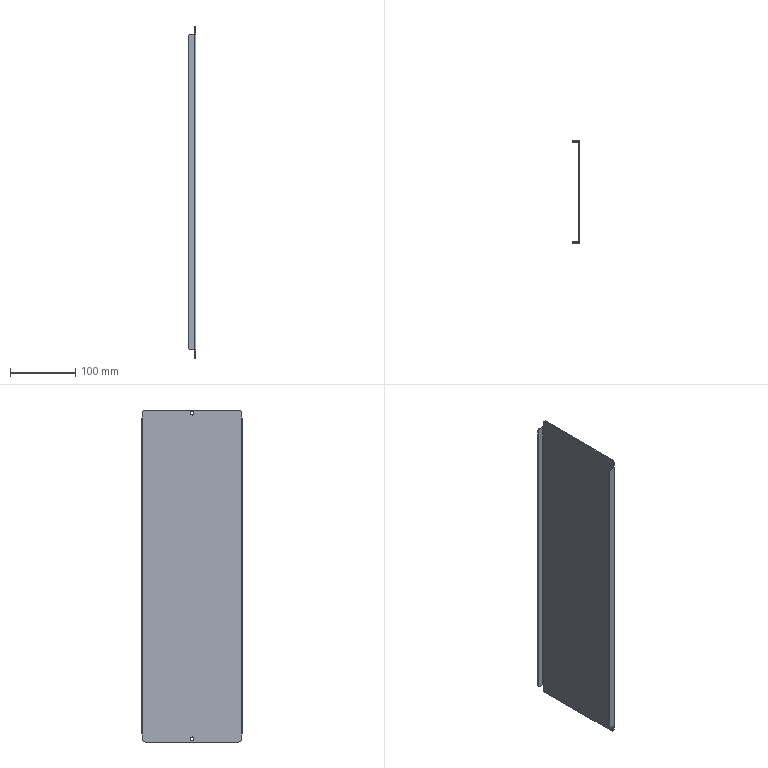Part | SolidWorks | 1 solid | 38 faces | box 12 x 156.2 x 510 mm | volume 133984 mm3 | plane 22 | cylinder 16 | commonest cylinder face diameters 10 x8 5.5 x4 0.2 x2 3.2 x2
STEP:
#1=CARTESIAN_POINT('',(-1.5,0.,247.25));
#2=VERTEX_POINT('',#1);
#3=CARTESIAN_POINT('',(-1.5,0.,252.75));
#4=VERTEX_POINT('',#3);
#5=CARTESIAN_POINT('',(-1.5,0.,250.));
#6=DIRECTION('',(-1.,0.,0.));
#7=DIRECTION('',(0.,0.,-1.));
#8=AXIS2_PLACEMENT_3D('',#5,#6,#7);
#9=CIRCLE('',#8,2.75);
#10=EDGE_CURVE('',#2,#4,#9,.T.);
#11=ORIENTED_EDGE('',*,*,#10,.T.);
#12=CARTESIAN_POINT('',(0.,0.,252.75));
#13=VERTEX_POINT('',#12);
#14=CARTESIAN_POINT('',(-12.001,0.,252.75));
#15=DIRECTION('',(1.,0.,0.));
#16=VECTOR('',#15,1000.);
#17=LINE('',#14,#16);
#18=EDGE_CURVE('',#4,#13,#17,.T.);
#19=ORIENTED_EDGE('',*,*,#18,.T.);
#20=CARTESIAN_POINT('',(0.,0.,247.25));
#21=VERTEX_POINT('',#20);
#22=CARTESIAN_POINT('',(0.,0.,250.));
#23=DIRECTION('',(1.,0.,0.));
#24=DIRECTION('',(0.,0.,-1.));
#25=AXIS2_PLACEMENT_3D('',#22,#23,#24);
#26=CIRCLE('',#25,2.75);
#27=EDGE_CURVE('',#13,#21,#26,.T.);
#28=ORIENTED_EDGE('',*,*,#27,.T.);
#29=CARTESIAN_POINT('',(-12.001,0.,247.25));
#30=DIRECTION('',(1.,0.,0.));
#31=VECTOR('',#30,1000.);
#32=LINE('',#29,#31);
#33=EDGE_CURVE('',#2,#21,#32,.T.);
#34=ORIENTED_EDGE('',*,*,#33,.F.);
#35=EDGE_LOOP('',(#11,#19,#28,#34));
#36=FACE_OUTER_BOUND('',#35,.T.);
#37=CARTESIAN_POINT('',(-12.001,0.,250.));
#38=DIRECTION('',(1.,0.,0.));
#39=DIRECTION('',(0.,0.,-1.));
#40=AXIS2_PLACEMENT_3D('',#37,#38,#39);
#41=CYLINDRICAL_SURFACE('',#40,2.75);
#42=ADVANCED_FACE('',(#36),#41,.F.);
#43=CARTESIAN_POINT('',(-1.5,0.,-252.75));
#44=VERTEX_POINT('',#43);
#45=CARTESIAN_POINT('',(-1.5,0.,-247.25));
#46=VERTEX_POINT('',#45);
#47=CARTESIAN_POINT('',(-1.5,0.,-250.));
#48=DIRECTION('',(-1.,0.,0.));
#49=DIRECTION('',(0.,0.,-1.));
#50=AXIS2_PLACEMENT_3D('',#47,#48,#49);
#51=CIRCLE('',#50,2.75);
#52=EDGE_CURVE('',#44,#46,#51,.T.);
#53=ORIENTED_EDGE('',*,*,#52,.T.);
#54=CARTESIAN_POINT('',(0.,0.,-247.25));
#55=VERTEX_POINT('',#54);
#56=CARTESIAN_POINT('',(-12.001,0.,-247.25));
#57=DIRECTION('',(1.,0.,0.));
#58=VECTOR('',#57,1000.);
#59=LINE('',#56,#58);
#60=EDGE_CURVE('',#46,#55,#59,.T.);
#61=ORIENTED_EDGE('',*,*,#60,.T.);
#62=CARTESIAN_POINT('',(0.,0.,-252.75));
#63=VERTEX_POINT('',#62);
#64=CARTESIAN_POINT('',(0.,0.,-250.));
#65=DIRECTION('',(1.,0.,0.));
#66=DIRECTION('',(0.,0.,1.));
#67=AXIS2_PLACEMENT_3D('',#64,#65,#66);
#68=CIRCLE('',#67,2.75);
#69=EDGE_CURVE('',#55,#63,#68,.T.);
#70=ORIENTED_EDGE('',*,*,#69,.T.);
#71=CARTESIAN_POINT('',(-12.001,0.,-252.75));
#72=DIRECTION('',(1.,0.,0.));
#73=VECTOR('',#72,1000.);
#74=LINE('',#71,#73);
#75=EDGE_CURVE('',#44,#63,#74,.T.);
#76=ORIENTED_EDGE('',*,*,#75,.F.);
#77=EDGE_LOOP('',(#53,#61,#70,#76));
#78=FACE_OUTER_BOUND('',#77,.T.);
#79=CARTESIAN_POINT('',(-12.001,0.,-250.));
#80=DIRECTION('',(1.,0.,0.));
#81=DIRECTION('',(0.,0.,-1.));
#82=AXIS2_PLACEMENT_3D('',#79,#80,#81);
#83=CYLINDRICAL_SURFACE('',#82,2.75);
#84=ADVANCED_FACE('',(#78),#83,.F.);
#85=CARTESIAN_POINT('',(0.,-76.5,250.));
#86=VERTEX_POINT('',#85);
#87=CARTESIAN_POINT('',(0.,-76.5,242.5));
#88=VERTEX_POINT('',#87);
#89=CARTESIAN_POINT('',(0.,-76.5,-255.));
#90=DIRECTION('',(0.,0.,-1.));
#91=VECTOR('',#90,1000.);
#92=LINE('',#89,#91);
#93=EDGE_CURVE('',#86,#88,#92,.T.);
#94=ORIENTED_EDGE('',*,*,#93,.F.);
#95=CARTESIAN_POINT('',(-1.5,-76.5,250.));
#96=VERTEX_POINT('',#95);
#97=CARTESIAN_POINT('',(-1.5,-76.5,250.));
#98=DIRECTION('',(-1.,0.,0.));
#99=VECTOR('',#98,1000.);
#100=LINE('',#97,#99);
#101=EDGE_CURVE('',#86,#96,#100,.T.);
#102=ORIENTED_EDGE('',*,*,#101,.T.);
#103=CARTESIAN_POINT('',(-1.5,-76.5,242.5));
#104=VERTEX_POINT('',#103);
#105=CARTESIAN_POINT('',(-1.5,-76.5,-255.));
#106=DIRECTION('',(0.,0.,-1.));
#107=VECTOR('',#106,1000.);
#108=LINE('',#105,#107);
#109=EDGE_CURVE('',#96,#104,#108,.T.);
#110=ORIENTED_EDGE('',*,*,#109,.T.);
#111=CARTESIAN_POINT('',(-1.5,-76.5,242.5));
#112=DIRECTION('',(1.,0.,0.));
#113=VECTOR('',#112,1000.);
#114=LINE('',#111,#113);
#115=EDGE_CURVE('',#104,#88,#114,.T.);
#116=ORIENTED_EDGE('',*,*,#115,.T.);
#117=EDGE_LOOP('',(#94,#102,#110,#116));
#118=FACE_OUTER_BOUND('',#117,.T.);
#119=CARTESIAN_POINT('',(-1.5,-76.5,-255.));
#120=DIRECTION('',(0.,-1.,0.));
#121=DIRECTION('',(0.,0.,-1.));
#122=AXIS2_PLACEMENT_3D('',#119,#120,#121);
#123=PLANE('',#122);
#124=ADVANCED_FACE('',(#118),#123,.T.);
#125=CARTESIAN_POINT('',(0.,76.5,-250.));
#126=VERTEX_POINT('',#125);
#127=CARTESIAN_POINT('',(0.,76.5,-242.5));
#128=VERTEX_POINT('',#127);
#129=CARTESIAN_POINT('',(0.,76.5,-255.));
#130=DIRECTION('',(0.,0.,1.));
#131=VECTOR('',#130,1000.);
#132=LINE('',#129,#131);
#133=EDGE_CURVE('',#126,#128,#132,.T.);
#134=ORIENTED_EDGE('',*,*,#133,.F.);
#135=CARTESIAN_POINT('',(-1.5,76.5,-250.));
#136=VERTEX_POINT('',#135);
#137=CARTESIAN_POINT('',(-1.5,76.5,-250.));
#138=DIRECTION('',(-1.,0.,0.));
#139=VECTOR('',#138,1000.);
#140=LINE('',#137,#139);
#141=EDGE_CURVE('',#126,#136,#140,.T.);
#142=ORIENTED_EDGE('',*,*,#141,.T.);
#143=CARTESIAN_POINT('',(-1.5,76.5,-242.5));
#144=VERTEX_POINT('',#143);
#145=CARTESIAN_POINT('',(-1.5,76.5,-255.));
#146=DIRECTION('',(0.,0.,1.));
#147=VECTOR('',#146,1000.);
#148=LINE('',#145,#147);
#149=EDGE_CURVE('',#136,#144,#148,.T.);
#150=ORIENTED_EDGE('',*,*,#149,.T.);
#151=CARTESIAN_POINT('',(-1.5,76.5,-242.5));
#152=DIRECTION('',(1.,0.,0.));
#153=VECTOR('',#152,1000.);
#154=LINE('',#151,#153);
#155=EDGE_CURVE('',#144,#128,#154,.T.);
#156=ORIENTED_EDGE('',*,*,#155,.T.);
#157=EDGE_LOOP('',(#134,#142,#150,#156));
#158=FACE_OUTER_BOUND('',#157,.T.);
#159=CARTESIAN_POINT('',(-1.5,76.5,-255.));
#160=DIRECTION('',(0.,1.,0.));
#161=DIRECTION('',(0.,0.,1.));
#162=AXIS2_PLACEMENT_3D('',#159,#160,#161);
#163=PLANE('',#162);
#164=ADVANCED_FACE('',(#158),#163,.T.);
#165=CARTESIAN_POINT('',(0.,71.5,255.));
#166=VERTEX_POINT('',#165);
#167=CARTESIAN_POINT('',(0.,-71.5,255.));
#168=VERTEX_POINT('',#167);
#169=CARTESIAN_POINT('',(0.,-76.5,255.));
#170=DIRECTION('',(0.,-1.,0.));
#171=VECTOR('',#170,1000.);
#172=LINE('',#169,#171);
#173=EDGE_CURVE('',#166,#168,#172,.T.);
#174=ORIENTED_EDGE('',*,*,#173,.F.);
#175=CARTESIAN_POINT('',(-1.5,71.5,255.));
#176=VERTEX_POINT('',#175);
#177=CARTESIAN_POINT('',(-1.5,71.5,255.));
#178=DIRECTION('',(-1.,0.,0.));
#179=VECTOR('',#178,1000.);
#180=LINE('',#177,#179);
#181=EDGE_CURVE('',#166,#176,#180,.T.);
#182=ORIENTED_EDGE('',*,*,#181,.T.);
#183=CARTESIAN_POINT('',(-1.5,-71.5,255.));
#184=VERTEX_POINT('',#183);
#185=CARTESIAN_POINT('',(-1.5,-76.5,255.));
#186=DIRECTION('',(0.,-1.,0.));
#187=VECTOR('',#186,1000.);
#188=LINE('',#185,#187);
#189=EDGE_CURVE('',#176,#184,#188,.T.);
#190=ORIENTED_EDGE('',*,*,#189,.T.);
#191=CARTESIAN_POINT('',(-1.5,-71.5,255.));
#192=DIRECTION('',(1.,0.,0.));
#193=VECTOR('',#192,1000.);
#194=LINE('',#191,#193);
#195=EDGE_CURVE('',#184,#168,#194,.T.);
#196=ORIENTED_EDGE('',*,*,#195,.T.);
#197=EDGE_LOOP('',(#174,#182,#190,#196));
#198=FACE_OUTER_BOUND('',#197,.T.);
#199=CARTESIAN_POINT('',(-1.5,-76.5,255.));
#200=DIRECTION('',(0.,0.,1.));
#201=DIRECTION('',(1.,0.,0.));
#202=AXIS2_PLACEMENT_3D('',#199,#200,#201);
#203=PLANE('',#202);
#204=ADVANCED_FACE('',(#198),#203,.T.);
#205=CARTESIAN_POINT('',(-1.5,76.5,242.5));
#206=VERTEX_POINT('',#205);
#207=CARTESIAN_POINT('',(-1.5,76.5,250.));
#208=VERTEX_POINT('',#207);
#209=CARTESIAN_POINT('',(-1.5,76.5,-255.));
#210=DIRECTION('',(0.,0.,1.));
#211=VECTOR('',#210,1000.);
#212=LINE('',#209,#211);
#213=EDGE_CURVE('',#206,#208,#212,.T.);
#214=ORIENTED_EDGE('',*,*,#213,.T.);
#215=CARTESIAN_POINT('',(0.,76.5,250.));
#216=VERTEX_POINT('',#215);
#217=CARTESIAN_POINT('',(-1.5,76.5,250.));
#218=DIRECTION('',(1.,0.,0.));
#219=VECTOR('',#218,1000.);
#220=LINE('',#217,#219);
#221=EDGE_CURVE('',#208,#216,#220,.T.);
#222=ORIENTED_EDGE('',*,*,#221,.T.);
#223=CARTESIAN_POINT('',(0.,76.5,242.5));
#224=VERTEX_POINT('',#223);
#225=CARTESIAN_POINT('',(0.,76.5,-255.));
#226=DIRECTION('',(0.,0.,1.));
#227=VECTOR('',#226,1000.);
#228=LINE('',#225,#227);
#229=EDGE_CURVE('',#224,#216,#228,.T.);
#230=ORIENTED_EDGE('',*,*,#229,.F.);
#231=CARTESIAN_POINT('',(-1.5,76.5,242.5));
#232=DIRECTION('',(1.,0.,0.));
#233=VECTOR('',#232,1000.);
#234=LINE('',#231,#233);
#235=EDGE_CURVE('',#206,#224,#234,.T.);
#236=ORIENTED_EDGE('',*,*,#235,.F.);
#237=EDGE_LOOP('',(#214,#222,#230,#236));
#238=FACE_OUTER_BOUND('',#237,.T.);
#239=CARTESIAN_POINT('',(-1.5,76.5,-255.));
#240=DIRECTION('',(0.,1.,0.));
#241=DIRECTION('',(0.,0.,1.));
#242=AXIS2_PLACEMENT_3D('',#239,#240,#241);
#243=PLANE('',#242);
#244=ADVANCED_FACE('',(#238),#243,.T.);
#245=CARTESIAN_POINT('',(0.,-71.5,-255.));
#246=VERTEX_POINT('',#245);
#247=CARTESIAN_POINT('',(0.,71.5,-255.));
#248=VERTEX_POINT('',#247);
#249=CARTESIAN_POINT('',(0.,-76.5,-255.));
#250=DIRECTION('',(0.,1.,0.));
#251=VECTOR('',#250,1000.);
#252=LINE('',#249,#251);
#253=EDGE_CURVE('',#246,#248,#252,.T.);
#254=ORIENTED_EDGE('',*,*,#253,.F.);
#255=CARTESIAN_POINT('',(-1.5,-71.5,-255.));
#256=VERTEX_POINT('',#255);
#257=CARTESIAN_POINT('',(-1.5,-71.5,-255.));
#258=DIRECTION('',(-1.,0.,0.));
#259=VECTOR('',#258,1000.);
#260=LINE('',#257,#259);
#261=EDGE_CURVE('',#246,#256,#260,.T.);
#262=ORIENTED_EDGE('',*,*,#261,.T.);
#263=CARTESIAN_POINT('',(-1.5,71.5,-255.));
#264=VERTEX_POINT('',#263);
#265=CARTESIAN_POINT('',(-1.5,-76.5,-255.));
#266=DIRECTION('',(0.,1.,0.));
#267=VECTOR('',#266,1000.);
#268=LINE('',#265,#267);
#269=EDGE_CURVE('',#256,#264,#268,.T.);
#270=ORIENTED_EDGE('',*,*,#269,.T.);
#271=CARTESIAN_POINT('',(-1.5,71.5,-255.));
#272=DIRECTION('',(1.,0.,0.));
#273=VECTOR('',#272,1000.);
#274=LINE('',#271,#273);
#275=EDGE_CURVE('',#264,#248,#274,.T.);
#276=ORIENTED_EDGE('',*,*,#275,.T.);
#277=EDGE_LOOP('',(#254,#262,#270,#276));
#278=FACE_OUTER_BOUND('',#277,.T.);
#279=CARTESIAN_POINT('',(-1.5,-76.5,-255.));
#280=DIRECTION('',(0.,0.,-1.));
#281=DIRECTION('',(-1.,0.,0.));
#282=AXIS2_PLACEMENT_3D('',#279,#280,#281);
#283=PLANE('',#282);
#284=ADVANCED_FACE('',(#278),#283,.T.);
#285=CARTESIAN_POINT('',(-1.5,-76.5,-242.5));
#286=VERTEX_POINT('',#285);
#287=CARTESIAN_POINT('',(-1.5,-76.5,-250.));
#288=VERTEX_POINT('',#287);
#289=CARTESIAN_POINT('',(-1.5,-76.5,-255.));
#290=DIRECTION('',(0.,0.,-1.));
#291=VECTOR('',#290,1000.);
#292=LINE('',#289,#291);
#293=EDGE_CURVE('',#286,#288,#292,.T.);
#294=ORIENTED_EDGE('',*,*,#293,.T.);
#295=CARTESIAN_POINT('',(0.,-76.5,-250.));
#296=VERTEX_POINT('',#295);
#297=CARTESIAN_POINT('',(-1.5,-76.5,-250.));
#298=DIRECTION('',(1.,0.,0.));
#299=VECTOR('',#298,1000.);
#300=LINE('',#297,#299);
#301=EDGE_CURVE('',#288,#296,#300,.T.);
#302=ORIENTED_EDGE('',*,*,#301,.T.);
#303=CARTESIAN_POINT('',(0.,-76.5,-242.5));
#304=VERTEX_POINT('',#303);
#305=CARTESIAN_POINT('',(0.,-76.5,-255.));
#306=DIRECTION('',(0.,0.,-1.));
#307=VECTOR('',#306,1000.);
#308=LINE('',#305,#307);
#309=EDGE_CURVE('',#304,#296,#308,.T.);
#310=ORIENTED_EDGE('',*,*,#309,.F.);
#311=CARTESIAN_POINT('',(-1.5,-76.5,-242.5));
#312=DIRECTION('',(1.,0.,0.));
#313=VECTOR('',#312,1000.);
#314=LINE('',#311,#313);
#315=EDGE_CURVE('',#286,#304,#314,.T.);
#316=ORIENTED_EDGE('',*,*,#315,.F.);
#317=EDGE_LOOP('',(#294,#302,#310,#316));
#318=FACE_OUTER_BOUND('',#317,.T.);
#319=CARTESIAN_POINT('',(-1.5,-76.5,-255.));
#320=DIRECTION('',(0.,-1.,0.));
#321=DIRECTION('',(0.,0.,-1.));
#322=AXIS2_PLACEMENT_3D('',#319,#320,#321);
#323=PLANE('',#322);
#324=ADVANCED_FACE('',(#318),#323,.T.);
#325=ORIENTED_EDGE('',*,*,#10,.F.);
#326=CARTESIAN_POINT('',(-1.5,0.,250.));
#327=DIRECTION('',(-1.,0.,0.));
#328=DIRECTION('',(0.,0.,-1.));
#329=AXIS2_PLACEMENT_3D('',#326,#327,#328);
#330=CIRCLE('',#329,2.75);
#331=EDGE_CURVE('',#4,#2,#330,.T.);
#332=ORIENTED_EDGE('',*,*,#331,.F.);
#333=EDGE_LOOP('',(#325,#332));
#334=FACE_BOUND('',#333,.T.);
#335=ORIENTED_EDGE('',*,*,#52,.F.);
#336=CARTESIAN_POINT('',(-1.5,0.,-250.));
#337=DIRECTION('',(-1.,0.,0.));
#338=DIRECTION('',(0.,0.,-1.));
#339=AXIS2_PLACEMENT_3D('',#336,#337,#338);
#340=CIRCLE('',#339,2.75);
#341=EDGE_CURVE('',#46,#44,#340,.T.);
#342=ORIENTED_EDGE('',*,*,#341,.F.);
#343=EDGE_LOOP('',(#335,#342));
#344=FACE_BOUND('',#343,.T.);
#345=ORIENTED_EDGE('',*,*,#189,.F.);
#346=CARTESIAN_POINT('',(-1.5,71.5,250.));
#347=DIRECTION('',(-1.,0.,0.));
#348=DIRECTION('',(0.,0.,-1.));
#349=AXIS2_PLACEMENT_3D('',#346,#347,#348);
#350=CIRCLE('',#349,5.);
#351=EDGE_CURVE('',#176,#208,#350,.T.);
#352=ORIENTED_EDGE('',*,*,#351,.T.);
#353=ORIENTED_EDGE('',*,*,#213,.F.);
#354=CARTESIAN_POINT('',(-1.5,76.5,-242.5));
#355=DIRECTION('',(0.,0.,1.));
#356=VECTOR('',#355,1000.);
#357=LINE('',#354,#356);
#358=EDGE_CURVE('',#144,#206,#357,.T.);
#359=ORIENTED_EDGE('',*,*,#358,.F.);
#360=ORIENTED_EDGE('',*,*,#149,.F.);
#361=CARTESIAN_POINT('',(-1.5,71.5,-250.));
#362=DIRECTION('',(-1.,0.,0.));
#363=DIRECTION('',(0.,0.,-1.));
#364=AXIS2_PLACEMENT_3D('',#361,#362,#363);
#365=CIRCLE('',#364,5.);
#366=EDGE_CURVE('',#136,#264,#365,.T.);
#367=ORIENTED_EDGE('',*,*,#366,.T.);
#368=ORIENTED_EDGE('',*,*,#269,.F.);
#369=CARTESIAN_POINT('',(-1.5,-71.5,-250.));
#370=DIRECTION('',(-1.,0.,0.));
#371=DIRECTION('',(0.,0.,-1.));
#372=AXIS2_PLACEMENT_3D('',#369,#370,#371);
#373=CIRCLE('',#372,5.);
#374=EDGE_CURVE('',#256,#288,#373,.T.);
#375=ORIENTED_EDGE('',*,*,#374,.T.);
#376=ORIENTED_EDGE('',*,*,#293,.F.);
#377=CARTESIAN_POINT('',(-1.5,-76.5,242.5));
#378=DIRECTION('',(0.,0.,-1.));
#379=VECTOR('',#378,1000.);
#380=LINE('',#377,#379);
#381=EDGE_CURVE('',#104,#286,#380,.T.);
#382=ORIENTED_EDGE('',*,*,#381,.F.);
#383=ORIENTED_EDGE('',*,*,#109,.F.);
#384=CARTESIAN_POINT('',(-1.5,-71.5,250.));
#385=DIRECTION('',(-1.,0.,0.));
#386=DIRECTION('',(0.,0.,-1.));
#387=AXIS2_PLACEMENT_3D('',#384,#385,#386);
#388=CIRCLE('',#387,5.);
#389=EDGE_CURVE('',#96,#184,#388,.T.);
#390=ORIENTED_EDGE('',*,*,#389,.T.);
#391=EDGE_LOOP('',(#345,#352,#353,#359,#360,#367,#368,#375,#376,#382,#383,#390));
#392=FACE_OUTER_BOUND('',#391,.T.);
#393=CARTESIAN_POINT('',(-1.5,0.,0.));
#394=DIRECTION('',(1.,0.,0.));
#395=DIRECTION('',(0.,0.,-1.));
#396=AXIS2_PLACEMENT_3D('',#393,#394,#395);
#397=PLANE('',#396);
#398=ADVANCED_FACE('',(#334,#344,#392),#397,.F.);
#399=CARTESIAN_POINT('',(0.,0.,250.));
#400=DIRECTION('',(1.,0.,0.));
#401=DIRECTION('',(0.,0.,-1.));
#402=AXIS2_PLACEMENT_3D('',#399,#400,#401);
#403=CIRCLE('',#402,2.75);
#404=EDGE_CURVE('',#21,#13,#403,.T.);
#405=ORIENTED_EDGE('',*,*,#404,.F.);
#406=ORIENTED_EDGE('',*,*,#27,.F.);
#407=EDGE_LOOP('',(#405,#406));
#408=FACE_BOUND('',#407,.T.);
#409=CARTESIAN_POINT('',(0.,0.,-250.));
#410=DIRECTION('',(1.,0.,0.));
#411=DIRECTION('',(0.,0.,1.));
#412=AXIS2_PLACEMENT_3D('',#409,#410,#411);
#413=CIRCLE('',#412,2.75);
#414=EDGE_CURVE('',#63,#55,#413,.T.);
#415=ORIENTED_EDGE('',*,*,#414,.F.);
#416=ORIENTED_EDGE('',*,*,#69,.F.);
#417=EDGE_LOOP('',(#415,#416));
#418=FACE_BOUND('',#417,.T.);
#419=ORIENTED_EDGE('',*,*,#229,.T.);
#420=CARTESIAN_POINT('',(0.,71.5,250.));
#421=DIRECTION('',(1.,0.,0.));
#422=DIRECTION('',(0.,0.,-1.));
#423=AXIS2_PLACEMENT_3D('',#420,#421,#422);
#424=CIRCLE('',#423,5.);
#425=EDGE_CURVE('',#216,#166,#424,.T.);
#426=ORIENTED_EDGE('',*,*,#425,.T.);
#427=ORIENTED_EDGE('',*,*,#173,.T.);
#428=CARTESIAN_POINT('',(0.,-71.5,250.));
#429=DIRECTION('',(1.,0.,0.));
#430=DIRECTION('',(0.,0.,-1.));
#431=AXIS2_PLACEMENT_3D('',#428,#429,#430);
#432=CIRCLE('',#431,5.);
#433=EDGE_CURVE('',#168,#86,#432,.T.);
#434=ORIENTED_EDGE('',*,*,#433,.T.);
#435=ORIENTED_EDGE('',*,*,#93,.T.);
#436=CARTESIAN_POINT('',(0.,-76.5,242.5));
#437=DIRECTION('',(0.,0.,-1.));
#438=VECTOR('',#437,1000.);
#439=LINE('',#436,#438);
#440=EDGE_CURVE('',#88,#304,#439,.T.);
#441=ORIENTED_EDGE('',*,*,#440,.T.);
#442=ORIENTED_EDGE('',*,*,#309,.T.);
#443=CARTESIAN_POINT('',(0.,-71.5,-250.));
#444=DIRECTION('',(1.,0.,0.));
#445=DIRECTION('',(0.,0.,-1.));
#446=AXIS2_PLACEMENT_3D('',#443,#444,#445);
#447=CIRCLE('',#446,5.);
#448=EDGE_CURVE('',#296,#246,#447,.T.);
#449=ORIENTED_EDGE('',*,*,#448,.T.);
#450=ORIENTED_EDGE('',*,*,#253,.T.);
#451=CARTESIAN_POINT('',(0.,71.5,-250.));
#452=DIRECTION('',(1.,0.,0.));
#453=DIRECTION('',(0.,0.,-1.));
#454=AXIS2_PLACEMENT_3D('',#451,#452,#453);
#455=CIRCLE('',#454,5.);
#456=EDGE_CURVE('',#248,#126,#455,.T.);
#457=ORIENTED_EDGE('',*,*,#456,.T.);
#458=ORIENTED_EDGE('',*,*,#133,.T.);
#459=CARTESIAN_POINT('',(0.,76.5,-242.5));
#460=DIRECTION('',(0.,0.,1.));
#461=VECTOR('',#460,1000.);
#462=LINE('',#459,#461);
#463=EDGE_CURVE('',#128,#224,#462,.T.);
#464=ORIENTED_EDGE('',*,*,#463,.T.);
#465=EDGE_LOOP('',(#419,#426,#427,#434,#435,#441,#442,#449,#450,#457,#458,#464));
#466=FACE_OUTER_BOUND('',#465,.T.);
#467=CARTESIAN_POINT('',(0.,0.,0.));
#468=DIRECTION('',(1.,0.,0.));
#469=DIRECTION('',(0.,0.,-1.));
#470=AXIS2_PLACEMENT_3D('',#467,#468,#469);
#471=PLANE('',#470);
#472=ADVANCED_FACE('',(#408,#418,#466),#471,.T.);
#473=CARTESIAN_POINT('',(-1.6,76.6,242.5));
#474=VERTEX_POINT('',#473);
#475=CARTESIAN_POINT('',(-1.6,78.1,242.5));
#476=VERTEX_POINT('',#475);
#477=CARTESIAN_POINT('',(-1.6,78.1,242.5));
#478=DIRECTION('',(0.,1.,0.));
#479=VECTOR('',#478,1000.);
#480=LINE('',#477,#479);
#481=EDGE_CURVE('',#474,#476,#480,.T.);
#482=ORIENTED_EDGE('',*,*,#481,.F.);
#483=CARTESIAN_POINT('',(-1.6,76.5,242.5));
#484=DIRECTION('',(0.,0.,1.));
#485=DIRECTION('',(-1.,0.,0.));
#486=AXIS2_PLACEMENT_3D('',#483,#484,#485);
#487=CIRCLE('',#486,0.1);
#488=EDGE_CURVE('',#206,#474,#487,.T.);
#489=ORIENTED_EDGE('',*,*,#488,.F.);
#490=ORIENTED_EDGE('',*,*,#235,.T.);
#491=CARTESIAN_POINT('',(-1.6,76.5,242.5));
#492=DIRECTION('',(0.,0.,1.));
#493=DIRECTION('',(-1.,0.,0.));
#494=AXIS2_PLACEMENT_3D('',#491,#492,#493);
#495=CIRCLE('',#494,1.6);
#496=EDGE_CURVE('',#224,#476,#495,.T.);
#497=ORIENTED_EDGE('',*,*,#496,.T.);
#498=EDGE_LOOP('',(#482,#489,#490,#497));
#499=FACE_OUTER_BOUND('',#498,.T.);
#500=CARTESIAN_POINT('',(-1.6,76.5,242.5));
#501=DIRECTION('',(0.,0.,1.));
#502=DIRECTION('',(1.,0.,0.));
#503=AXIS2_PLACEMENT_3D('',#500,#501,#502);
#504=PLANE('',#503);
#505=ADVANCED_FACE('',(#499),#504,.T.);
#506=CARTESIAN_POINT('',(-1.6,76.6,-242.5));
#507=VERTEX_POINT('',#506);
#508=CARTESIAN_POINT('',(-1.6,76.5,-242.5));
#509=DIRECTION('',(0.,0.,-1.));
#510=DIRECTION('',(-1.,0.,0.));
#511=AXIS2_PLACEMENT_3D('',#508,#509,#510);
#512=CIRCLE('',#511,0.1);
#513=EDGE_CURVE('',#507,#144,#512,.T.);
#514=ORIENTED_EDGE('',*,*,#513,.F.);
#515=CARTESIAN_POINT('',(-1.6,78.1,-242.5));
#516=VERTEX_POINT('',#515);
#517=CARTESIAN_POINT('',(-1.6,76.6,-242.5));
#518=DIRECTION('',(0.,1.,0.));
#519=VECTOR('',#518,1000.);
#520=LINE('',#517,#519);
#521=EDGE_CURVE('',#507,#516,#520,.T.);
#522=ORIENTED_EDGE('',*,*,#521,.T.);
#523=CARTESIAN_POINT('',(-1.6,76.5,-242.5));
#524=DIRECTION('',(0.,0.,-1.));
#525=DIRECTION('',(-1.,0.,0.));
#526=AXIS2_PLACEMENT_3D('',#523,#524,#525);
#527=CIRCLE('',#526,1.6);
#528=EDGE_CURVE('',#516,#128,#527,.T.);
#529=ORIENTED_EDGE('',*,*,#528,.T.);
#530=ORIENTED_EDGE('',*,*,#155,.F.);
#531=EDGE_LOOP('',(#514,#522,#529,#530));
#532=FACE_OUTER_BOUND('',#531,.T.);
#533=CARTESIAN_POINT('',(-1.6,76.5,-242.5));
#534=DIRECTION('',(0.,0.,1.));
#535=DIRECTION('',(1.,0.,0.));
#536=AXIS2_PLACEMENT_3D('',#533,#534,#535);
#537=PLANE('',#536);
#538=ADVANCED_FACE('',(#532),#537,.F.);
#539=ORIENTED_EDGE('',*,*,#463,.F.);
#540=ORIENTED_EDGE('',*,*,#528,.F.);
#541=CARTESIAN_POINT('',(-1.6,78.1,242.5));
#542=DIRECTION('',(0.,0.,1.));
#543=VECTOR('',#542,1000.);
#544=LINE('',#541,#543);
#545=EDGE_CURVE('',#516,#476,#544,.T.);
#546=ORIENTED_EDGE('',*,*,#545,.T.);
#547=ORIENTED_EDGE('',*,*,#496,.F.);
#548=EDGE_LOOP('',(#539,#540,#546,#547));
#549=FACE_OUTER_BOUND('',#548,.T.);
#550=CARTESIAN_POINT('',(-1.6,76.5,-242.5));
#551=DIRECTION('',(0.,0.,-1.));
#552=DIRECTION('',(0.,1.,0.));
#553=AXIS2_PLACEMENT_3D('',#550,#551,#552);
#554=CYLINDRICAL_SURFACE('',#553,1.6);
#555=ADVANCED_FACE('',(#549),#554,.T.);
#556=ORIENTED_EDGE('',*,*,#358,.T.);
#557=ORIENTED_EDGE('',*,*,#488,.T.);
#558=CARTESIAN_POINT('',(-1.6,76.6,242.5));
#559=DIRECTION('',(0.,0.,-1.));
#560=VECTOR('',#559,1000.);
#561=LINE('',#558,#560);
#562=EDGE_CURVE('',#474,#507,#561,.T.);
#563=ORIENTED_EDGE('',*,*,#562,.T.);
#564=ORIENTED_EDGE('',*,*,#513,.T.);
#565=EDGE_LOOP('',(#556,#557,#563,#564));
#566=FACE_OUTER_BOUND('',#565,.T.);
#567=CARTESIAN_POINT('',(-1.6,76.5,-242.5));
#568=DIRECTION('',(0.,0.,-1.));
#569=DIRECTION('',(0.,1.,0.));
#570=AXIS2_PLACEMENT_3D('',#567,#568,#569);
#571=CYLINDRICAL_SURFACE('',#570,0.1);
#572=ADVANCED_FACE('',(#566),#571,.F.);
#573=CARTESIAN_POINT('',(-7.,76.6,-242.5));
#574=VERTEX_POINT('',#573);
#575=CARTESIAN_POINT('',(-12.,76.6,-242.5));
#576=DIRECTION('',(-1.,0.,0.));
#577=VECTOR('',#576,1000.);
#578=LINE('',#575,#577);
#579=EDGE_CURVE('',#507,#574,#578,.T.);
#580=ORIENTED_EDGE('',*,*,#579,.T.);
#581=CARTESIAN_POINT('',(-7.,78.1,-242.5));
#582=VERTEX_POINT('',#581);
#583=CARTESIAN_POINT('',(-7.,78.1,-242.5));
#584=DIRECTION('',(0.,1.,0.));
#585=VECTOR('',#584,1000.);
#586=LINE('',#583,#585);
#587=EDGE_CURVE('',#574,#582,#586,.T.);
#588=ORIENTED_EDGE('',*,*,#587,.T.);
#589=CARTESIAN_POINT('',(0.,78.1,-242.5));
#590=DIRECTION('',(-1.,0.,0.));
#591=VECTOR('',#590,1000.);
#592=LINE('',#589,#591);
#593=EDGE_CURVE('',#516,#582,#592,.T.);
#594=ORIENTED_EDGE('',*,*,#593,.F.);
#595=ORIENTED_EDGE('',*,*,#521,.F.);
#596=EDGE_LOOP('',(#580,#588,#594,#595));
#597=FACE_OUTER_BOUND('',#596,.T.);
#598=CARTESIAN_POINT('',(-12.,78.1,-242.5));
#599=DIRECTION('',(0.,0.,1.));
#600=DIRECTION('',(0.,-1.,0.));
#601=AXIS2_PLACEMENT_3D('',#598,#599,#600);
#602=PLANE('',#601);
#603=ADVANCED_FACE('',(#597),#602,.F.);
#604=CARTESIAN_POINT('',(-7.,78.1,242.5));
#605=VERTEX_POINT('',#604);
#606=CARTESIAN_POINT('',(0.,78.1,242.5));
#607=DIRECTION('',(1.,0.,0.));
#608=VECTOR('',#607,1000.);
#609=LINE('',#606,#608);
#610=EDGE_CURVE('',#605,#476,#609,.T.);
#611=ORIENTED_EDGE('',*,*,#610,.F.);
#612=CARTESIAN_POINT('',(-7.,76.6,242.5));
#613=VERTEX_POINT('',#612);
#614=CARTESIAN_POINT('',(-7.,78.1,242.5));
#615=DIRECTION('',(0.,-1.,0.));
#616=VECTOR('',#615,1000.);
#617=LINE('',#614,#616);
#618=EDGE_CURVE('',#605,#613,#617,.T.);
#619=ORIENTED_EDGE('',*,*,#618,.T.);
#620=CARTESIAN_POINT('',(-1.5,76.6,242.5));
#621=DIRECTION('',(1.,0.,0.));
#622=VECTOR('',#621,1000.);
#623=LINE('',#620,#622);
#624=EDGE_CURVE('',#613,#474,#623,.T.);
#625=ORIENTED_EDGE('',*,*,#624,.T.);
#626=ORIENTED_EDGE('',*,*,#481,.T.);
#627=EDGE_LOOP('',(#611,#619,#625,#626));
#628=FACE_OUTER_BOUND('',#627,.T.);
#629=CARTESIAN_POINT('',(-1.5,78.1,242.5));
#630=DIRECTION('',(0.,0.,-1.));
#631=DIRECTION('',(0.,1.,0.));
#632=AXIS2_PLACEMENT_3D('',#629,#630,#631);
#633=PLANE('',#632);
#634=ADVANCED_FACE('',(#628),#633,.F.);
#635=CARTESIAN_POINT('',(-12.,78.1,-237.5));
#636=VERTEX_POINT('',#635);
#637=CARTESIAN_POINT('',(-12.,78.1,237.5));
#638=VERTEX_POINT('',#637);
#639=CARTESIAN_POINT('',(-12.,78.1,0.));
#640=DIRECTION('',(0.,0.,1.));
#641=VECTOR('',#640,1000.);
#642=LINE('',#639,#641);
#643=EDGE_CURVE('',#636,#638,#642,.T.);
#644=ORIENTED_EDGE('',*,*,#643,.T.);
#645=CARTESIAN_POINT('',(-7.,78.1,237.5));
#646=DIRECTION('',(0.,1.,0.));
#647=DIRECTION('',(1.,0.,0.));
#648=AXIS2_PLACEMENT_3D('',#645,#646,#647);
#649=CIRCLE('',#648,5.);
#650=EDGE_CURVE('',#638,#605,#649,.T.);
#651=ORIENTED_EDGE('',*,*,#650,.T.);
#652=ORIENTED_EDGE('',*,*,#610,.T.);
#653=ORIENTED_EDGE('',*,*,#545,.F.);
#654=ORIENTED_EDGE('',*,*,#593,.T.);
#655=CARTESIAN_POINT('',(-7.,78.1,-237.5));
#656=DIRECTION('',(0.,1.,0.));
#657=DIRECTION('',(1.,0.,0.));
#658=AXIS2_PLACEMENT_3D('',#655,#656,#657);
#659=CIRCLE('',#658,5.);
#660=EDGE_CURVE('',#582,#636,#659,.T.);
#661=ORIENTED_EDGE('',*,*,#660,.T.);
#662=EDGE_LOOP('',(#644,#651,#652,#653,#654,#661));
#663=FACE_OUTER_BOUND('',#662,.T.);
#664=CARTESIAN_POINT('',(0.,78.1,0.));
#665=DIRECTION('',(0.,-1.,0.));
#666=DIRECTION('',(1.,0.,0.));
#667=AXIS2_PLACEMENT_3D('',#664,#665,#666);
#668=PLANE('',#667);
#669=ADVANCED_FACE('',(#663),#668,.F.);
#670=ORIENTED_EDGE('',*,*,#624,.F.);
#671=CARTESIAN_POINT('',(-12.,76.6,237.5));
#672=VERTEX_POINT('',#671);
#673=CARTESIAN_POINT('',(-7.,76.6,237.5));
#674=DIRECTION('',(0.,-1.,0.));
#675=DIRECTION('',(1.,0.,0.));
#676=AXIS2_PLACEMENT_3D('',#673,#674,#675);
#677=CIRCLE('',#676,5.);
#678=EDGE_CURVE('',#613,#672,#677,.T.);
#679=ORIENTED_EDGE('',*,*,#678,.T.);
#680=CARTESIAN_POINT('',(-12.,76.6,-237.5));
#681=VERTEX_POINT('',#680);
#682=CARTESIAN_POINT('',(-12.,76.6,242.5));
#683=DIRECTION('',(0.,0.,1.));
#684=VECTOR('',#683,1000.);
#685=LINE('',#682,#684);
#686=EDGE_CURVE('',#681,#672,#685,.T.);
#687=ORIENTED_EDGE('',*,*,#686,.F.);
#688=CARTESIAN_POINT('',(-7.,76.6,-237.5));
#689=DIRECTION('',(0.,-1.,0.));
#690=DIRECTION('',(1.,0.,0.));
#691=AXIS2_PLACEMENT_3D('',#688,#689,#690);
#692=CIRCLE('',#691,5.);
#693=EDGE_CURVE('',#681,#574,#692,.T.);
#694=ORIENTED_EDGE('',*,*,#693,.T.);
#695=ORIENTED_EDGE('',*,*,#579,.F.);
#696=ORIENTED_EDGE('',*,*,#562,.F.);
#697=EDGE_LOOP('',(#670,#679,#687,#694,#695,#696));
#698=FACE_OUTER_BOUND('',#697,.T.);
#699=CARTESIAN_POINT('',(0.,76.6,0.));
#700=DIRECTION('',(0.,-1.,0.));
#701=DIRECTION('',(1.,0.,0.));
#702=AXIS2_PLACEMENT_3D('',#699,#700,#701);
#703=PLANE('',#702);
#704=ADVANCED_FACE('',(#698),#703,.T.);
#705=ORIENTED_EDGE('',*,*,#686,.T.);
#706=CARTESIAN_POINT('',(-12.,78.1,237.5));
#707=DIRECTION('',(0.,1.,0.));
#708=VECTOR('',#707,1000.);
#709=LINE('',#706,#708);
#710=EDGE_CURVE('',#672,#638,#709,.T.);
#711=ORIENTED_EDGE('',*,*,#710,.T.);
#712=ORIENTED_EDGE('',*,*,#643,.F.);
#713=CARTESIAN_POINT('',(-12.,78.1,-237.5));
#714=DIRECTION('',(0.,-1.,0.));
#715=VECTOR('',#714,1000.);
#716=LINE('',#713,#715);
#717=EDGE_CURVE('',#636,#681,#716,.T.);
#718=ORIENTED_EDGE('',*,*,#717,.T.);
#719=EDGE_LOOP('',(#705,#711,#712,#718));
#720=FACE_OUTER_BOUND('',#719,.T.);
#721=CARTESIAN_POINT('',(-12.,78.1,242.5));
#722=DIRECTION('',(1.,0.,0.));
#723=DIRECTION('',(0.,1.,0.));
#724=AXIS2_PLACEMENT_3D('',#721,#722,#723);
#725=PLANE('',#724);
#726=ADVANCED_FACE('',(#720),#725,.F.);
#727=CARTESIAN_POINT('',(-1.6,-76.6,-242.5));
#728=VERTEX_POINT('',#727);
#729=CARTESIAN_POINT('',(-1.6,-78.1,-242.5));
#730=VERTEX_POINT('',#729);
#731=CARTESIAN_POINT('',(-1.6,-78.1,-242.5));
#732=DIRECTION('',(0.,-1.,0.));
#733=VECTOR('',#732,1000.);
#734=LINE('',#731,#733);
#735=EDGE_CURVE('',#728,#730,#734,.T.);
#736=ORIENTED_EDGE('',*,*,#735,.F.);
#737=CARTESIAN_POINT('',(-1.6,-76.5,-242.5));
#738=DIRECTION('',(0.,0.,-1.));
#739=DIRECTION('',(1.,0.,0.));
#740=AXIS2_PLACEMENT_3D('',#737,#738,#739);
#741=CIRCLE('',#740,0.1);
#742=EDGE_CURVE('',#286,#728,#741,.T.);
#743=ORIENTED_EDGE('',*,*,#742,.F.);
#744=ORIENTED_EDGE('',*,*,#315,.T.);
#745=CARTESIAN_POINT('',(-1.6,-76.5,-242.5));
#746=DIRECTION('',(0.,0.,-1.));
#747=DIRECTION('',(1.,0.,0.));
#748=AXIS2_PLACEMENT_3D('',#745,#746,#747);
#749=CIRCLE('',#748,1.6);
#750=EDGE_CURVE('',#304,#730,#749,.T.);
#751=ORIENTED_EDGE('',*,*,#750,.T.);
#752=EDGE_LOOP('',(#736,#743,#744,#751));
#753=FACE_OUTER_BOUND('',#752,.T.);
#754=CARTESIAN_POINT('',(-1.6,-76.5,-242.5));
#755=DIRECTION('',(0.,0.,-1.));
#756=DIRECTION('',(-1.,0.,0.));
#757=AXIS2_PLACEMENT_3D('',#754,#755,#756);
#758=PLANE('',#757);
#759=ADVANCED_FACE('',(#753),#758,.T.);
#760=CARTESIAN_POINT('',(-1.6,-76.6,242.5));
#761=VERTEX_POINT('',#760);
#762=CARTESIAN_POINT('',(-1.6,-76.5,242.5));
#763=DIRECTION('',(0.,0.,1.));
#764=DIRECTION('',(1.,0.,0.));
#765=AXIS2_PLACEMENT_3D('',#762,#763,#764);
#766=CIRCLE('',#765,0.1);
#767=EDGE_CURVE('',#761,#104,#766,.T.);
#768=ORIENTED_EDGE('',*,*,#767,.F.);
#769=CARTESIAN_POINT('',(-1.6,-78.1,242.5));
#770=VERTEX_POINT('',#769);
#771=CARTESIAN_POINT('',(-1.6,-76.6,242.5));
#772=DIRECTION('',(0.,-1.,0.));
#773=VECTOR('',#772,1000.);
#774=LINE('',#771,#773);
#775=EDGE_CURVE('',#761,#770,#774,.T.);
#776=ORIENTED_EDGE('',*,*,#775,.T.);
#777=CARTESIAN_POINT('',(-1.6,-76.5,242.5));
#778=DIRECTION('',(0.,0.,1.));
#779=DIRECTION('',(1.,0.,0.));
#780=AXIS2_PLACEMENT_3D('',#777,#778,#779);
#781=CIRCLE('',#780,1.6);
#782=EDGE_CURVE('',#770,#88,#781,.T.);
#783=ORIENTED_EDGE('',*,*,#782,.T.);
#784=ORIENTED_EDGE('',*,*,#115,.F.);
#785=EDGE_LOOP('',(#768,#776,#783,#784));
#786=FACE_OUTER_BOUND('',#785,.T.);
#787=CARTESIAN_POINT('',(-1.6,-76.5,242.5));
#788=DIRECTION('',(0.,0.,-1.));
#789=DIRECTION('',(-1.,0.,0.));
#790=AXIS2_PLACEMENT_3D('',#787,#788,#789);
#791=PLANE('',#790);
#792=ADVANCED_FACE('',(#786),#791,.F.);
#793=ORIENTED_EDGE('',*,*,#440,.F.);
#794=ORIENTED_EDGE('',*,*,#782,.F.);
#795=CARTESIAN_POINT('',(-1.6,-78.1,-242.5));
#796=DIRECTION('',(0.,0.,-1.));
#797=VECTOR('',#796,1000.);
#798=LINE('',#795,#797);
#799=EDGE_CURVE('',#770,#730,#798,.T.);
#800=ORIENTED_EDGE('',*,*,#799,.T.);
#801=ORIENTED_EDGE('',*,*,#750,.F.);
#802=EDGE_LOOP('',(#793,#794,#800,#801));
#803=FACE_OUTER_BOUND('',#802,.T.);
#804=CARTESIAN_POINT('',(-1.6,-76.5,242.5));
#805=DIRECTION('',(0.,0.,1.));
#806=DIRECTION('',(0.,-1.,0.));
#807=AXIS2_PLACEMENT_3D('',#804,#805,#806);
#808=CYLINDRICAL_SURFACE('',#807,1.6);
#809=ADVANCED_FACE('',(#803),#808,.T.);
#810=ORIENTED_EDGE('',*,*,#381,.T.);
#811=ORIENTED_EDGE('',*,*,#742,.T.);
#812=CARTESIAN_POINT('',(-1.6,-76.6,-242.5));
#813=DIRECTION('',(0.,0.,1.));
#814=VECTOR('',#813,1000.);
#815=LINE('',#812,#814);
#816=EDGE_CURVE('',#728,#761,#815,.T.);
#817=ORIENTED_EDGE('',*,*,#816,.T.);
#818=ORIENTED_EDGE('',*,*,#767,.T.);
#819=EDGE_LOOP('',(#810,#811,#817,#818));
#820=FACE_OUTER_BOUND('',#819,.T.);
#821=CARTESIAN_POINT('',(-1.6,-76.5,242.5));
#822=DIRECTION('',(0.,0.,1.));
#823=DIRECTION('',(0.,-1.,0.));
#824=AXIS2_PLACEMENT_3D('',#821,#822,#823);
#825=CYLINDRICAL_SURFACE('',#824,0.1);
#826=ADVANCED_FACE('',(#820),#825,.F.);
#827=CARTESIAN_POINT('',(-7.,-76.6,242.5));
#828=VERTEX_POINT('',#827);
#829=CARTESIAN_POINT('',(-12.,-76.6,242.5));
#830=DIRECTION('',(-1.,0.,0.));
#831=VECTOR('',#830,1000.);
#832=LINE('',#829,#831);
#833=EDGE_CURVE('',#761,#828,#832,.T.);
#834=ORIENTED_EDGE('',*,*,#833,.T.);
#835=CARTESIAN_POINT('',(-7.,-78.1,242.5));
#836=VERTEX_POINT('',#835);
#837=CARTESIAN_POINT('',(-7.,-78.1,242.5));
#838=DIRECTION('',(0.,-1.,0.));
#839=VECTOR('',#838,1000.);
#840=LINE('',#837,#839);
#841=EDGE_CURVE('',#828,#836,#840,.T.);
#842=ORIENTED_EDGE('',*,*,#841,.T.);
#843=CARTESIAN_POINT('',(0.,-78.1,242.5));
#844=DIRECTION('',(-1.,0.,0.));
#845=VECTOR('',#844,1000.);
#846=LINE('',#843,#845);
#847=EDGE_CURVE('',#770,#836,#846,.T.);
#848=ORIENTED_EDGE('',*,*,#847,.F.);
#849=ORIENTED_EDGE('',*,*,#775,.F.);
#850=EDGE_LOOP('',(#834,#842,#848,#849));
#851=FACE_OUTER_BOUND('',#850,.T.);
#852=CARTESIAN_POINT('',(-12.,-78.1,242.5));
#853=DIRECTION('',(0.,0.,-1.));
#854=DIRECTION('',(0.,1.,0.));
#855=AXIS2_PLACEMENT_3D('',#852,#853,#854);
#856=PLANE('',#855);
#857=ADVANCED_FACE('',(#851),#856,.F.);
#858=CARTESIAN_POINT('',(-7.,-78.1,-242.5));
#859=VERTEX_POINT('',#858);
#860=CARTESIAN_POINT('',(0.,-78.1,-242.5));
#861=DIRECTION('',(1.,0.,0.));
#862=VECTOR('',#861,1000.);
#863=LINE('',#860,#862);
#864=EDGE_CURVE('',#859,#730,#863,.T.);
#865=ORIENTED_EDGE('',*,*,#864,.F.);
#866=CARTESIAN_POINT('',(-7.,-76.6,-242.5));
#867=VERTEX_POINT('',#866);
#868=CARTESIAN_POINT('',(-7.,-78.1,-242.5));
#869=DIRECTION('',(0.,1.,0.));
#870=VECTOR('',#869,1000.);
#871=LINE('',#868,#870);
#872=EDGE_CURVE('',#859,#867,#871,.T.);
#873=ORIENTED_EDGE('',*,*,#872,.T.);
#874=CARTESIAN_POINT('',(-1.5,-76.6,-242.5));
#875=DIRECTION('',(1.,0.,0.));
#876=VECTOR('',#875,1000.);
#877=LINE('',#874,#876);
#878=EDGE_CURVE('',#867,#728,#877,.T.);
#879=ORIENTED_EDGE('',*,*,#878,.T.);
#880=ORIENTED_EDGE('',*,*,#735,.T.);
#881=EDGE_LOOP('',(#865,#873,#879,#880));
#882=FACE_OUTER_BOUND('',#881,.T.);
#883=CARTESIAN_POINT('',(-1.5,-78.1,-242.5));
#884=DIRECTION('',(0.,0.,1.));
#885=DIRECTION('',(0.,-1.,0.));
#886=AXIS2_PLACEMENT_3D('',#883,#884,#885);
#887=PLANE('',#886);
#888=ADVANCED_FACE('',(#882),#887,.F.);
#889=ORIENTED_EDGE('',*,*,#847,.T.);
#890=CARTESIAN_POINT('',(-12.,-78.1,237.5));
#891=VERTEX_POINT('',#890);
#892=CARTESIAN_POINT('',(-7.,-78.1,237.5));
#893=DIRECTION('',(0.,-1.,0.));
#894=DIRECTION('',(-1.,0.,0.));
#895=AXIS2_PLACEMENT_3D('',#892,#893,#894);
#896=CIRCLE('',#895,5.);
#897=EDGE_CURVE('',#836,#891,#896,.T.);
#898=ORIENTED_EDGE('',*,*,#897,.T.);
#899=CARTESIAN_POINT('',(-12.,-78.1,-237.5));
#900=VERTEX_POINT('',#899);
#901=CARTESIAN_POINT('',(-12.,-78.1,0.));
#902=DIRECTION('',(0.,0.,-1.));
#903=VECTOR('',#902,1000.);
#904=LINE('',#901,#903);
#905=EDGE_CURVE('',#891,#900,#904,.T.);
#906=ORIENTED_EDGE('',*,*,#905,.T.);
#907=CARTESIAN_POINT('',(-7.,-78.1,-237.5));
#908=DIRECTION('',(0.,-1.,0.));
#909=DIRECTION('',(-1.,0.,0.));
#910=AXIS2_PLACEMENT_3D('',#907,#908,#909);
#911=CIRCLE('',#910,5.);
#912=EDGE_CURVE('',#900,#859,#911,.T.);
#913=ORIENTED_EDGE('',*,*,#912,.T.);
#914=ORIENTED_EDGE('',*,*,#864,.T.);
#915=ORIENTED_EDGE('',*,*,#799,.F.);
#916=EDGE_LOOP('',(#889,#898,#906,#913,#914,#915));
#917=FACE_OUTER_BOUND('',#916,.T.);
#918=CARTESIAN_POINT('',(0.,-78.1,0.));
#919=DIRECTION('',(0.,1.,0.));
#920=DIRECTION('',(-1.,0.,0.));
#921=AXIS2_PLACEMENT_3D('',#918,#919,#920);
#922=PLANE('',#921);
#923=ADVANCED_FACE('',(#917),#922,.F.);
#924=CARTESIAN_POINT('',(-12.,-76.6,237.5));
#925=VERTEX_POINT('',#924);
#926=CARTESIAN_POINT('',(-12.,-76.6,-237.5));
#927=VERTEX_POINT('',#926);
#928=CARTESIAN_POINT('',(-12.,-76.6,-242.5));
#929=DIRECTION('',(0.,0.,-1.));
#930=VECTOR('',#929,1000.);
#931=LINE('',#928,#930);
#932=EDGE_CURVE('',#925,#927,#931,.T.);
#933=ORIENTED_EDGE('',*,*,#932,.F.);
#934=CARTESIAN_POINT('',(-7.,-76.6,237.5));
#935=DIRECTION('',(0.,1.,0.));
#936=DIRECTION('',(-1.,0.,0.));
#937=AXIS2_PLACEMENT_3D('',#934,#935,#936);
#938=CIRCLE('',#937,5.);
#939=EDGE_CURVE('',#925,#828,#938,.T.);
#940=ORIENTED_EDGE('',*,*,#939,.T.);
#941=ORIENTED_EDGE('',*,*,#833,.F.);
#942=ORIENTED_EDGE('',*,*,#816,.F.);
#943=ORIENTED_EDGE('',*,*,#878,.F.);
#944=CARTESIAN_POINT('',(-7.,-76.6,-237.5));
#945=DIRECTION('',(0.,1.,0.));
#946=DIRECTION('',(-1.,0.,0.));
#947=AXIS2_PLACEMENT_3D('',#944,#945,#946);
#948=CIRCLE('',#947,5.);
#949=EDGE_CURVE('',#867,#927,#948,.T.);
#950=ORIENTED_EDGE('',*,*,#949,.T.);
#951=EDGE_LOOP('',(#933,#940,#941,#942,#943,#950));
#952=FACE_OUTER_BOUND('',#951,.T.);
#953=CARTESIAN_POINT('',(0.,-76.6,0.));
#954=DIRECTION('',(0.,1.,0.));
#955=DIRECTION('',(-1.,0.,0.));
#956=AXIS2_PLACEMENT_3D('',#953,#954,#955);
#957=PLANE('',#956);
#958=ADVANCED_FACE('',(#952),#957,.T.);
#959=ORIENTED_EDGE('',*,*,#905,.F.);
#960=CARTESIAN_POINT('',(-12.,-78.1,237.5));
#961=DIRECTION('',(0.,1.,0.));
#962=VECTOR('',#961,1000.);
#963=LINE('',#960,#962);
#964=EDGE_CURVE('',#891,#925,#963,.T.);
#965=ORIENTED_EDGE('',*,*,#964,.T.);
#966=ORIENTED_EDGE('',*,*,#932,.T.);
#967=CARTESIAN_POINT('',(-12.,-78.1,-237.5));
#968=DIRECTION('',(0.,-1.,0.));
#969=VECTOR('',#968,1000.);
#970=LINE('',#967,#969);
#971=EDGE_CURVE('',#927,#900,#970,.T.);
#972=ORIENTED_EDGE('',*,*,#971,.T.);
#973=EDGE_LOOP('',(#959,#965,#966,#972));
#974=FACE_OUTER_BOUND('',#973,.T.);
#975=CARTESIAN_POINT('',(-12.,-78.1,-242.5));
#976=DIRECTION('',(1.,0.,0.));
#977=DIRECTION('',(0.,1.,0.));
#978=AXIS2_PLACEMENT_3D('',#975,#976,#977);
#979=PLANE('',#978);
#980=ADVANCED_FACE('',(#974),#979,.F.);
#981=ORIENTED_EDGE('',*,*,#351,.F.);
#982=ORIENTED_EDGE('',*,*,#181,.F.);
#983=ORIENTED_EDGE('',*,*,#425,.F.);
#984=ORIENTED_EDGE('',*,*,#221,.F.);
#985=EDGE_LOOP('',(#981,#982,#983,#984));
#986=FACE_OUTER_BOUND('',#985,.T.);
#987=CARTESIAN_POINT('',(-1.5,71.5,250.));
#988=DIRECTION('',(1.,0.,0.));
#989=DIRECTION('',(0.,0.,-1.));
#990=AXIS2_PLACEMENT_3D('',#987,#988,#989);
#991=CYLINDRICAL_SURFACE('',#990,5.);
#992=ADVANCED_FACE('',(#986),#991,.T.);
#993=ORIENTED_EDGE('',*,*,#650,.F.);
#994=ORIENTED_EDGE('',*,*,#710,.F.);
#995=ORIENTED_EDGE('',*,*,#678,.F.);
#996=ORIENTED_EDGE('',*,*,#618,.F.);
#997=EDGE_LOOP('',(#993,#994,#995,#996));
#998=FACE_OUTER_BOUND('',#997,.T.);
#999=CARTESIAN_POINT('',(-7.,78.1,237.5));
#1000=DIRECTION('',(0.,-1.,0.));
#1001=DIRECTION('',(1.,0.,0.));
#1002=AXIS2_PLACEMENT_3D('',#999,#1000,#1001);
#1003=CYLINDRICAL_SURFACE('',#1002,5.);
#1004=ADVANCED_FACE('',(#998),#1003,.T.);
#1005=ORIENTED_EDGE('',*,*,#897,.F.);
#1006=ORIENTED_EDGE('',*,*,#841,.F.);
#1007=ORIENTED_EDGE('',*,*,#939,.F.);
#1008=ORIENTED_EDGE('',*,*,#964,.F.);
#1009=EDGE_LOOP('',(#1005,#1006,#1007,#1008));
#1010=FACE_OUTER_BOUND('',#1009,.T.);
#1011=CARTESIAN_POINT('',(-7.,-78.1,237.5));
#1012=DIRECTION('',(0.,1.,0.));
#1013=DIRECTION('',(-1.,0.,0.));
#1014=AXIS2_PLACEMENT_3D('',#1011,#1012,#1013);
#1015=CYLINDRICAL_SURFACE('',#1014,5.);
#1016=ADVANCED_FACE('',(#1010),#1015,.T.);
#1017=ORIENTED_EDGE('',*,*,#389,.F.);
#1018=ORIENTED_EDGE('',*,*,#101,.F.);
#1019=ORIENTED_EDGE('',*,*,#433,.F.);
#1020=ORIENTED_EDGE('',*,*,#195,.F.);
#1021=EDGE_LOOP('',(#1017,#1018,#1019,#1020));
#1022=FACE_OUTER_BOUND('',#1021,.T.);
#1023=CARTESIAN_POINT('',(-1.5,-71.5,250.));
#1024=DIRECTION('',(1.,0.,0.));
#1025=DIRECTION('',(0.,0.,-1.));
#1026=AXIS2_PLACEMENT_3D('',#1023,#1024,#1025);
#1027=CYLINDRICAL_SURFACE('',#1026,5.);
#1028=ADVANCED_FACE('',(#1022),#1027,.T.);
#1029=ORIENTED_EDGE('',*,*,#374,.F.);
#1030=ORIENTED_EDGE('',*,*,#261,.F.);
#1031=ORIENTED_EDGE('',*,*,#448,.F.);
#1032=ORIENTED_EDGE('',*,*,#301,.F.);
#1033=EDGE_LOOP('',(#1029,#1030,#1031,#1032));
#1034=FACE_OUTER_BOUND('',#1033,.T.);
#1035=CARTESIAN_POINT('',(-1.5,-71.5,-250.));
#1036=DIRECTION('',(1.,0.,0.));
#1037=DIRECTION('',(0.,0.,-1.));
#1038=AXIS2_PLACEMENT_3D('',#1035,#1036,#1037);
#1039=CYLINDRICAL_SURFACE('',#1038,5.);
#1040=ADVANCED_FACE('',(#1034),#1039,.T.);
#1041=ORIENTED_EDGE('',*,*,#912,.F.);
#1042=ORIENTED_EDGE('',*,*,#971,.F.);
#1043=ORIENTED_EDGE('',*,*,#949,.F.);
#1044=ORIENTED_EDGE('',*,*,#872,.F.);
#1045=EDGE_LOOP('',(#1041,#1042,#1043,#1044));
#1046=FACE_OUTER_BOUND('',#1045,.T.);
#1047=CARTESIAN_POINT('',(-7.,-78.1,-237.5));
#1048=DIRECTION('',(0.,1.,0.));
#1049=DIRECTION('',(-1.,0.,0.));
#1050=AXIS2_PLACEMENT_3D('',#1047,#1048,#1049);
#1051=CYLINDRICAL_SURFACE('',#1050,5.);
#1052=ADVANCED_FACE('',(#1046),#1051,.T.);
#1053=ORIENTED_EDGE('',*,*,#366,.F.);
#1054=ORIENTED_EDGE('',*,*,#141,.F.);
#1055=ORIENTED_EDGE('',*,*,#456,.F.);
#1056=ORIENTED_EDGE('',*,*,#275,.F.);
#1057=EDGE_LOOP('',(#1053,#1054,#1055,#1056));
#1058=FACE_OUTER_BOUND('',#1057,.T.);
#1059=CARTESIAN_POINT('',(-1.5,71.5,-250.));
#1060=DIRECTION('',(1.,0.,0.));
#1061=DIRECTION('',(0.,0.,-1.));
#1062=AXIS2_PLACEMENT_3D('',#1059,#1060,#1061);
#1063=CYLINDRICAL_SURFACE('',#1062,5.);
#1064=ADVANCED_FACE('',(#1058),#1063,.T.);
#1065=ORIENTED_EDGE('',*,*,#660,.F.);
#1066=ORIENTED_EDGE('',*,*,#587,.F.);
#1067=ORIENTED_EDGE('',*,*,#693,.F.);
#1068=ORIENTED_EDGE('',*,*,#717,.F.);
#1069=EDGE_LOOP('',(#1065,#1066,#1067,#1068));
#1070=FACE_OUTER_BOUND('',#1069,.T.);
#1071=CARTESIAN_POINT('',(-7.,78.1,-237.5));
#1072=DIRECTION('',(0.,-1.,0.));
#1073=DIRECTION('',(1.,0.,0.));
#1074=AXIS2_PLACEMENT_3D('',#1071,#1072,#1073);
#1075=CYLINDRICAL_SURFACE('',#1074,5.);
#1076=ADVANCED_FACE('',(#1070),#1075,.T.);
#1077=ORIENTED_EDGE('',*,*,#60,.F.);
#1078=ORIENTED_EDGE('',*,*,#341,.T.);
#1079=ORIENTED_EDGE('',*,*,#75,.T.);
#1080=ORIENTED_EDGE('',*,*,#414,.T.);
#1081=EDGE_LOOP('',(#1077,#1078,#1079,#1080));
#1082=FACE_OUTER_BOUND('',#1081,.T.);
#1083=CARTESIAN_POINT('',(-12.001,0.,-250.));
#1084=DIRECTION('',(1.,0.,0.));
#1085=DIRECTION('',(0.,0.,-1.));
#1086=AXIS2_PLACEMENT_3D('',#1083,#1084,#1085);
#1087=CYLINDRICAL_SURFACE('',#1086,2.75);
#1088=ADVANCED_FACE('',(#1082),#1087,.F.);
#1089=ORIENTED_EDGE('',*,*,#18,.F.);
#1090=ORIENTED_EDGE('',*,*,#331,.T.);
#1091=ORIENTED_EDGE('',*,*,#33,.T.);
#1092=ORIENTED_EDGE('',*,*,#404,.T.);
#1093=EDGE_LOOP('',(#1089,#1090,#1091,#1092));
#1094=FACE_OUTER_BOUND('',#1093,.T.);
#1095=CARTESIAN_POINT('',(-12.001,0.,250.));
#1096=DIRECTION('',(1.,0.,0.));
#1097=DIRECTION('',(0.,0.,-1.));
#1098=AXIS2_PLACEMENT_3D('',#1095,#1096,#1097);
#1099=CYLINDRICAL_SURFACE('',#1098,2.75);
#1100=ADVANCED_FACE('',(#1094),#1099,.F.);
#1101=CLOSED_SHELL('',(#42,#84,#124,#164,#204,#244,#284,#324,#398,#472,#505,#538,#555,#572,#603,#634,#669,#704,#726,#759,#792,#809,#826,#857,#888,#923,#958,#980,#992,#1004,#1016,#1028,#1040,#1052,#1064,#1076,#1088,#1100));
#1102=MANIFOLD_SOLID_BREP('',#1101);
#1103=CARTESIAN_POINT('',(0.,0.,0.));
#1104=DIRECTION('',(0.,0.,1.));
#1105=DIRECTION('',(1.,0.,0.));
#1106=AXIS2_PLACEMENT_3D('',#1103,#1104,#1105);
#1107=(LENGTH_UNIT()NAMED_UNIT(*)SI_UNIT(.MILLI.,.METRE.));
#1108=UNCERTAINTY_MEASURE_WITH_UNIT(LENGTH_MEASURE(0.00001),#1107,'','');
#1109=(NAMED_UNIT(*)PLANE_ANGLE_UNIT()SI_UNIT($,.RADIAN.));
#1110=(NAMED_UNIT(*)SI_UNIT($,.STERADIAN.)SOLID_ANGLE_UNIT());
#1111=(GEOMETRIC_REPRESENTATION_CONTEXT(3)GLOBAL_UNCERTAINTY_ASSIGNED_CONTEXT((#1108))GLOBAL_UNIT_ASSIGNED_CONTEXT((#1107,#1109,#1110))REPRESENTATION_CONTEXT('',''));
#1112=ADVANCED_BREP_SHAPE_REPRESENTATION('',(#1102,#1106),#1111);